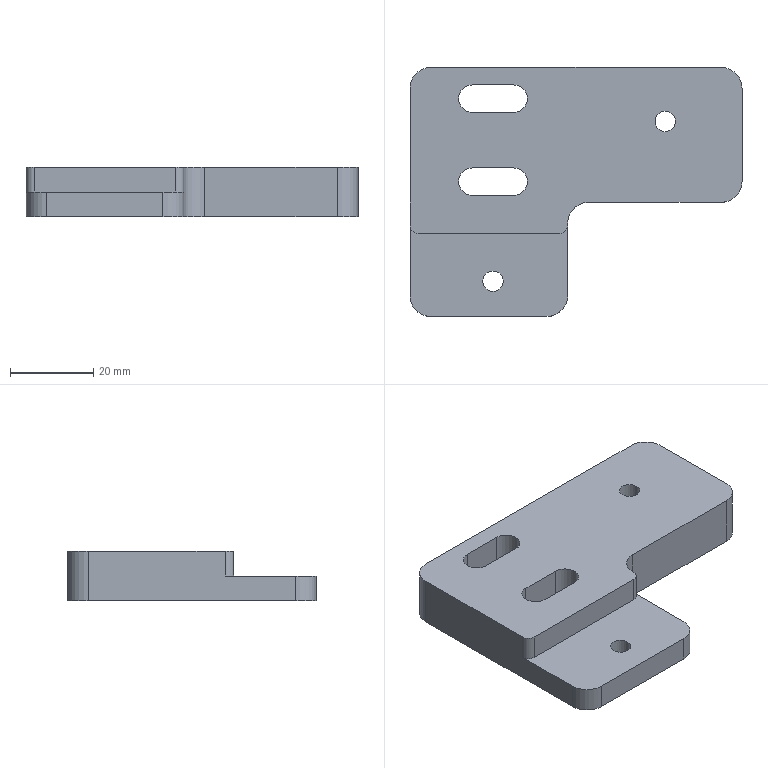NC program | NX | posted with a generic post | part box 80 x 60 x 12 mm
Lines 2097 to 2921 of 5338:
(ZLEVEL_PROFILE , TOOL : D4)
N4168 T11 M6
N4170 G54
N4172 G17 G0 G90 X-14.065 Y21.599 S9500 M3
N4174 G43 Z30. H11
N4176 Z1.5
N4178 G94 G1 X-13.892 Y21.801 Z1.486 F1650.
N4180 X-13.737 Y22.152 Z1.466
N4182 X-13.69 Y22.534 Z1.446
N4184 X-13.757 Y22.913 Z1.426
N4186 X-13.896 Y23.205 Z1.409
N4188 X-14.146 Y23.494 Z1.389
N4190 X-14.47 Y23.698 Z1.369
N4192 X-14.838 Y23.8 Z1.349
N4194 X-25.162 Z0.808
N4196 X-25.53 Y23.698 Z0.787
N4198 X-25.854 Y23.494 Z0.767
N4200 X-26.104 Y23.205 Z0.747
N4202 X-26.243 Y22.913 Z0.73
N4204 X-26.31 Y22.534 Z0.71
N4206 X-26.263 Y22.152 Z0.69
N4208 X-26.108 Y21.801 Z0.67
N4210 X-25.857 Y21.509 Z0.65
N4212 X-25.532 Y21.303 Z0.63
N4214 X-25.162 Y21.2 Z0.61
N4216 X-14.838 Z0.069
N4218 X-14.468 Y21.303 Z0.048
N4220 X-14.143 Y21.509 Z0.028
N4222 X-13.892 Y21.801 Z0.008
N4224 X-13.737 Y22.152 Z-0.012
N4226 X-13.69 Y22.534 Z-0.032
N4228 X-13.757 Y22.913 Z-0.052
N4230 X-13.896 Y23.205 Z-0.069
N4232 X-14.146 Y23.494 Z-0.089
N4234 X-14.47 Y23.698 Z-0.109
N4236 X-14.838 Y23.8 Z-0.129
N4238 X-20. Z-0.4
N4240 X-25.
N4242 G3 X-26.3 Y22.5 R1.3
N4244 X-25. Y21.2 R1.3
N4246 G1 X-15.
N4248 G3 X-13.7 Y22.5 R1.3
N4250 X-15. Y23.8 R1.3
N4252 G1 X-20.
N4254 X-24.789 Z-0.491
N4256 X-24.929 Z-0.493
N4258 X-25.07 Y23.79 Z-0.496
N4260 X-25.209 Y23.777 Z-0.499
N4262 X-25.346 Y23.746 Z-0.501
N4264 X-25.5 Y23.692 Z-0.504
N4266 X-25.606 Y23.643 Z-0.507
N4268 X-25.697 Y23.589 Z-0.509
N4270 X-25.742 Y23.562 Z-0.51
N4272 X-25.837 Y23.486 Z-0.512
N4274 X-25.963 Y23.362 Z-0.515
N4276 X-26.03 Y23.283 Z-0.517
N4278 X-26.113 Y23.162 Z-0.52
N4280 X-26.173 Y23.043 Z-0.523
N4282 X-26.238 Y22.871 Z-0.526
N4284 X-26.265 Y22.778 Z-0.528
N4286 X-26.286 Y22.637 Z-0.531
N4288 X-26.292 Y22.5 Z-0.533
N4290 X-26.28 Y22.323 Z-0.537
N4292 X-26.265 Y22.222 Z-0.539
N4294 X-26.224 Y22.085 Z-0.541
N4296 X-26.173 Y21.957 Z-0.544
N4298 X-26.093 Y21.809 Z-0.547
N4300 X-26.03 Y21.717 Z-0.549
N4302 X-25.925 Y21.598 Z-0.552
N4304 X-25.837 Y21.514 Z-0.555
N4306 X-25.709 Y21.417 Z-0.558
N4308 X-25.606 Y21.357 Z-0.56
N4310 X-25.452 Y21.289 Z-0.563
N4312 X-25.346 Y21.254 Z-0.565
N4314 X-25.209 Y21.223 Z-0.568
N4316 X-25.07 Y21.21 Z-0.571
N4318 X-24.929 Y21.2 Z-0.573
N4320 X-24.789 Z-0.576
N4322 X-15.211 Z-0.757
N4324 X-15.071 Z-0.76
N4326 X-14.93 Y21.21 Z-0.763
N4328 X-14.791 Y21.223 Z-0.765
N4330 X-14.654 Y21.254 Z-0.768
N4332 X-14.48 Y21.308 Z-0.771
N4334 X-14.391 Y21.351 Z-0.773
N4336 X-14.158 Y21.509 Z-0.779
N4338 X-14.094 Y21.568 Z-0.78
N4340 X-14.029 Y21.635 Z-0.782
N4342 X-13.97 Y21.717 Z-0.784
N4344 X-13.891 Y21.832 Z-0.787
N4346 X-13.827 Y21.957 Z-0.789
N4348 X-13.765 Y22.119 Z-0.793
N4350 X-13.735 Y22.222 Z-0.795
N4352 X-13.714 Y22.36 Z-0.797
N4354 X-13.7 Y22.5 Z-0.8
N4356 G3 X-15. Y23.8 R1.3
N4358 G1 X-20.
N4360 X-24.789 Z-0.891
N4362 X-24.929 Z-0.893
N4364 X-25.07 Y23.79 Z-0.896
N4366 X-25.209 Y23.777 Z-0.899
N4368 X-25.346 Y23.746 Z-0.901
N4370 X-25.5 Y23.692 Z-0.904
N4372 X-25.606 Y23.643 Z-0.907
N4374 X-25.697 Y23.589 Z-0.909
N4376 X-25.742 Y23.562 Z-0.91
N4378 X-25.837 Y23.486 Z-0.912
N4380 X-25.963 Y23.362 Z-0.915
N4382 X-26.03 Y23.283 Z-0.917
N4384 X-26.113 Y23.162 Z-0.92
N4386 X-26.173 Y23.043 Z-0.923
N4388 X-26.238 Y22.871 Z-0.926
N4390 X-26.265 Y22.778 Z-0.928
N4392 X-26.286 Y22.637 Z-0.931
N4394 X-26.292 Y22.5 Z-0.933
N4396 X-26.28 Y22.323 Z-0.937
N4398 X-26.265 Y22.222 Z-0.939
N4400 X-26.224 Y22.085 Z-0.941
N4402 X-26.173 Y21.957 Z-0.944
N4404 X-26.093 Y21.809 Z-0.947
N4406 X-26.03 Y21.717 Z-0.949
N4408 X-25.925 Y21.598 Z-0.952
N4410 X-25.837 Y21.514 Z-0.955
N4412 X-25.709 Y21.417 Z-0.958
N4414 X-25.606 Y21.357 Z-0.96
N4416 X-25.452 Y21.289 Z-0.963
N4418 X-25.346 Y21.254 Z-0.965
N4420 X-25.209 Y21.223 Z-0.968
N4422 X-25.07 Y21.21 Z-0.971
N4424 X-24.929 Y21.2 Z-0.973
N4426 X-24.789 Z-0.976
N4428 X-15.211 Z-1.157
N4430 X-15.071 Z-1.16
N4432 X-14.93 Y21.21 Z-1.163
N4434 X-14.791 Y21.223 Z-1.165
N4436 X-14.654 Y21.254 Z-1.168
N4438 X-14.48 Y21.308 Z-1.171
N4440 X-14.391 Y21.351 Z-1.173
N4442 X-14.158 Y21.509 Z-1.179
N4444 X-14.094 Y21.568 Z-1.18
N4446 X-14.029 Y21.635 Z-1.182
N4448 X-13.97 Y21.717 Z-1.184
N4450 X-13.891 Y21.832 Z-1.187
N4452 X-13.827 Y21.957 Z-1.189
N4454 X-13.765 Y22.119 Z-1.193
N4456 X-13.735 Y22.222 Z-1.195
N4458 X-13.714 Y22.36 Z-1.197
N4460 X-13.7 Y22.5 Z-1.2
N4462 G3 X-15. Y23.8 R1.3
N4464 G1 X-20.
N4466 X-24.789 Z-1.291
N4468 X-24.929 Z-1.293
N4470 X-25.07 Y23.79 Z-1.296
N4472 X-25.209 Y23.777 Z-1.299
N4474 X-25.346 Y23.746 Z-1.301
N4476 X-25.5 Y23.692 Z-1.304
N4478 X-25.606 Y23.643 Z-1.307
N4480 X-25.697 Y23.589 Z-1.309
N4482 X-25.742 Y23.562 Z-1.31
N4484 X-25.837 Y23.486 Z-1.312
N4486 X-25.962 Y23.362 Z-1.315
N4488 X-26.03 Y23.283 Z-1.317
N4490 X-26.113 Y23.162 Z-1.32
N4492 X-26.173 Y23.043 Z-1.323
N4494 X-26.238 Y22.871 Z-1.326
N4496 X-26.265 Y22.778 Z-1.328
N4498 X-26.286 Y22.637 Z-1.331
N4500 X-26.292 Y22.5 Z-1.333
N4502 X-26.28 Y22.323 Z-1.337
N4504 X-26.265 Y22.222 Z-1.339
N4506 X-26.224 Y22.085 Z-1.341
N4508 X-26.173 Y21.957 Z-1.344
N4510 X-26.093 Y21.809 Z-1.347
N4512 X-26.03 Y21.717 Z-1.349
N4514 X-25.925 Y21.598 Z-1.352
N4516 X-25.837 Y21.514 Z-1.355
N4518 X-25.709 Y21.417 Z-1.358
N4520 X-25.606 Y21.357 Z-1.36
N4522 X-25.452 Y21.289 Z-1.363
N4524 X-25.346 Y21.254 Z-1.365
N4526 X-25.209 Y21.223 Z-1.368
N4528 X-25.07 Y21.21 Z-1.371
N4530 X-24.929 Y21.2 Z-1.373
N4532 X-24.789 Z-1.376
N4534 X-15.211 Z-1.557
N4536 X-15.071 Z-1.56
N4538 X-14.93 Y21.21 Z-1.563
N4540 X-14.791 Y21.223 Z-1.565
N4542 X-14.654 Y21.254 Z-1.568
N4544 X-14.48 Y21.308 Z-1.571
N4546 X-14.391 Y21.351 Z-1.573
N4548 X-14.158 Y21.509 Z-1.579
N4550 X-14.094 Y21.568 Z-1.58
N4552 X-14.029 Y21.635 Z-1.582
N4554 X-13.97 Y21.717 Z-1.584
N4556 X-13.891 Y21.832 Z-1.587
N4558 X-13.827 Y21.957 Z-1.589
N4560 X-13.765 Y22.119 Z-1.593
N4562 X-13.735 Y22.222 Z-1.595
N4564 X-13.714 Y22.36 Z-1.597
N4566 X-13.7 Y22.5 Z-1.6
N4568 G3 X-15. Y23.8 R1.3
N4570 G1 X-20.
N4572 X-24.789 Z-1.691
N4574 X-24.929 Z-1.693
N4576 X-25.07 Y23.79 Z-1.696
N4578 X-25.209 Y23.777 Z-1.699
N4580 X-25.346 Y23.746 Z-1.701
N4582 X-25.5 Y23.692 Z-1.704
N4584 X-25.606 Y23.643 Z-1.707
N4586 X-25.697 Y23.589 Z-1.709
N4588 X-25.742 Y23.562 Z-1.71
N4590 X-25.837 Y23.486 Z-1.712
N4592 X-25.962 Y23.362 Z-1.715
N4594 X-26.03 Y23.283 Z-1.717
N4596 X-26.113 Y23.162 Z-1.72
N4598 X-26.173 Y23.043 Z-1.723
N4600 X-26.238 Y22.871 Z-1.726
N4602 X-26.265 Y22.778 Z-1.728
N4604 X-26.286 Y22.637 Z-1.731
N4606 X-26.292 Y22.5 Z-1.733
N4608 X-26.28 Y22.323 Z-1.737
N4610 X-26.265 Y22.222 Z-1.739
N4612 X-26.224 Y22.085 Z-1.741
N4614 X-26.173 Y21.957 Z-1.744
N4616 X-26.093 Y21.809 Z-1.747
N4618 X-26.03 Y21.717 Z-1.749
N4620 X-25.925 Y21.598 Z-1.752
N4622 X-25.837 Y21.514 Z-1.755
N4624 X-25.709 Y21.417 Z-1.758
N4626 X-25.606 Y21.357 Z-1.76
N4628 X-25.452 Y21.289 Z-1.763
N4630 X-25.346 Y21.254 Z-1.765
N4632 X-25.209 Y21.223 Z-1.768
N4634 X-25.07 Y21.21 Z-1.771
N4636 X-24.929 Y21.2 Z-1.773
N4638 X-24.789 Z-1.776
N4640 X-15.211 Z-1.957
N4642 X-15.071 Z-1.96
N4644 X-14.93 Y21.21 Z-1.963
N4646 X-14.791 Y21.223 Z-1.965
N4648 X-14.654 Y21.254 Z-1.968
N4650 X-14.48 Y21.308 Z-1.971
N4652 X-14.391 Y21.351 Z-1.973
N4654 X-14.158 Y21.509 Z-1.979
N4656 X-14.094 Y21.568 Z-1.98
N4658 X-14.029 Y21.635 Z-1.982
N4660 X-13.97 Y21.717 Z-1.984
N4662 X-13.891 Y21.832 Z-1.987
N4664 X-13.827 Y21.957 Z-1.989
N4666 X-13.765 Y22.119 Z-1.993
N4668 X-13.735 Y22.222 Z-1.995
N4670 X-13.714 Y22.36 Z-1.997
N4672 X-13.7 Y22.5 Z-2.
N4674 G3 X-15. Y23.8 R1.3
N4676 G1 X-20.
N4678 X-24.789 Z-2.091
N4680 X-24.929 Z-2.093
N4682 X-25.07 Y23.79 Z-2.096
N4684 X-25.209 Y23.777 Z-2.099
N4686 X-25.346 Y23.746 Z-2.101
N4688 X-25.5 Y23.692 Z-2.104
N4690 X-25.606 Y23.643 Z-2.107
N4692 X-25.697 Y23.589 Z-2.109
N4694 X-25.742 Y23.562 Z-2.11
N4696 X-25.837 Y23.486 Z-2.112
N4698 X-25.962 Y23.362 Z-2.115
N4700 X-26.03 Y23.283 Z-2.117
N4702 X-26.113 Y23.162 Z-2.12
N4704 X-26.173 Y23.043 Z-2.123
N4706 X-26.238 Y22.871 Z-2.126
N4708 X-26.265 Y22.778 Z-2.128
N4710 X-26.286 Y22.637 Z-2.131
N4712 X-26.292 Y22.5 Z-2.133
N4714 X-26.28 Y22.323 Z-2.137
N4716 X-26.265 Y22.222 Z-2.139
N4718 X-26.224 Y22.085 Z-2.141
N4720 X-26.173 Y21.957 Z-2.144
N4722 X-26.093 Y21.809 Z-2.147
N4724 X-26.03 Y21.717 Z-2.149
N4726 X-25.925 Y21.598 Z-2.152
N4728 X-25.837 Y21.514 Z-2.155
N4730 X-25.709 Y21.417 Z-2.158
N4732 X-25.606 Y21.357 Z-2.16
N4734 X-25.452 Y21.289 Z-2.163
N4736 X-25.346 Y21.254 Z-2.165
N4738 X-25.209 Y21.223 Z-2.168
N4740 X-25.07 Y21.21 Z-2.171
N4742 X-24.929 Y21.2 Z-2.173
N4744 X-24.789 Z-2.176
N4746 X-15.211 Z-2.357
N4748 X-15.071 Z-2.36
N4750 X-14.93 Y21.21 Z-2.363
N4752 X-14.791 Y21.223 Z-2.365
N4754 X-14.654 Y21.254 Z-2.368
N4756 X-14.48 Y21.308 Z-2.371
N4758 X-14.391 Y21.351 Z-2.373
N4760 X-14.158 Y21.509 Z-2.379
N4762 X-14.094 Y21.568 Z-2.38
N4764 X-14.03 Y21.635 Z-2.382
N4766 X-13.97 Y21.717 Z-2.384
N4768 X-13.891 Y21.832 Z-2.387
N4770 X-13.827 Y21.957 Z-2.389
N4772 X-13.765 Y22.119 Z-2.393
N4774 X-13.735 Y22.222 Z-2.395
N4776 X-13.714 Y22.36 Z-2.397
N4778 X-13.7 Y22.5 Z-2.4
N4780 G3 X-15. Y23.8 R1.3
N4782 G1 X-20.
N4784 X-24.789 Z-2.491
N4786 X-24.929 Z-2.493
N4788 X-25.07 Y23.79 Z-2.496
N4790 X-25.209 Y23.777 Z-2.499
N4792 X-25.346 Y23.746 Z-2.501
N4794 X-25.5 Y23.692 Z-2.504
N4796 X-25.606 Y23.643 Z-2.507
N4798 X-25.697 Y23.589 Z-2.509
N4800 X-25.742 Y23.562 Z-2.51
N4802 X-25.837 Y23.486 Z-2.512
N4804 X-25.962 Y23.362 Z-2.515
N4806 X-26.03 Y23.283 Z-2.517
N4808 X-26.113 Y23.162 Z-2.52
N4810 X-26.173 Y23.043 Z-2.523
N4812 X-26.238 Y22.871 Z-2.526
N4814 X-26.265 Y22.778 Z-2.528
N4816 X-26.286 Y22.637 Z-2.531
N4818 X-26.292 Y22.5 Z-2.533
N4820 X-26.28 Y22.323 Z-2.537
N4822 X-26.265 Y22.222 Z-2.539
N4824 X-26.224 Y22.085 Z-2.541
N4826 X-26.173 Y21.957 Z-2.544
N4828 X-26.093 Y21.809 Z-2.547
N4830 X-26.03 Y21.717 Z-2.549
N4832 X-25.925 Y21.598 Z-2.552
N4834 X-25.837 Y21.514 Z-2.555
N4836 X-25.709 Y21.417 Z-2.558
N4838 X-25.606 Y21.357 Z-2.56
N4840 X-25.452 Y21.289 Z-2.563
N4842 X-25.346 Y21.254 Z-2.565
N4844 X-25.209 Y21.223 Z-2.568
N4846 X-25.07 Y21.21 Z-2.571
N4848 X-24.929 Y21.2 Z-2.573
N4850 X-24.789 Z-2.576
N4852 X-15.211 Z-2.757
N4854 X-15.071 Z-2.76
N4856 X-14.93 Y21.21 Z-2.763
N4858 X-14.791 Y21.223 Z-2.765
N4860 X-14.654 Y21.254 Z-2.768
N4862 X-14.48 Y21.308 Z-2.771
N4864 X-14.391 Y21.351 Z-2.773
N4866 X-14.158 Y21.509 Z-2.779
N4868 X-14.094 Y21.567 Z-2.78
N4870 X-14.03 Y21.635 Z-2.782
N4872 X-13.97 Y21.717 Z-2.784
N4874 X-13.891 Y21.832 Z-2.787
N4876 X-13.827 Y21.957 Z-2.789
N4878 X-13.765 Y22.119 Z-2.793
N4880 X-13.735 Y22.222 Z-2.795
N4882 X-13.714 Y22.36 Z-2.797
N4884 X-13.7 Y22.5 Z-2.8
N4886 G3 X-15. Y23.8 R1.3
N4888 G1 X-20.
N4890 X-24.789 Z-2.891
N4892 X-24.929 Z-2.893
N4894 X-25.07 Y23.79 Z-2.896
N4896 X-25.209 Y23.777 Z-2.899
N4898 X-25.346 Y23.746 Z-2.901
N4900 X-25.5 Y23.692 Z-2.904
N4902 X-25.606 Y23.643 Z-2.907
N4904 X-25.742 Y23.562 Z-2.91
N4906 X-25.837 Y23.486 Z-2.912
N4908 X-25.962 Y23.362 Z-2.915
N4910 X-26.03 Y23.283 Z-2.917
N4912 X-26.113 Y23.162 Z-2.92
N4914 X-26.173 Y23.043 Z-2.923
N4916 X-26.238 Y22.871 Z-2.926
N4918 X-26.265 Y22.778 Z-2.928
N4920 X-26.286 Y22.637 Z-2.931
N4922 X-26.292 Y22.5 Z-2.933
N4924 X-26.28 Y22.323 Z-2.937
N4926 X-26.265 Y22.222 Z-2.939
N4928 X-26.224 Y22.085 Z-2.941
N4930 X-26.173 Y21.957 Z-2.944
N4932 X-26.093 Y21.809 Z-2.947
N4934 X-26.03 Y21.717 Z-2.949
N4936 X-25.925 Y21.598 Z-2.952
N4938 X-25.837 Y21.514 Z-2.955
N4940 X-25.709 Y21.417 Z-2.958
N4942 X-25.606 Y21.357 Z-2.96
N4944 X-25.452 Y21.289 Z-2.963
N4946 X-25.346 Y21.254 Z-2.965
N4948 X-25.209 Y21.223 Z-2.968
N4950 X-25.07 Y21.21 Z-2.971
N4952 X-24.929 Y21.2 Z-2.973
N4954 X-24.789 Z-2.976
N4956 X-15.211 Z-3.157
N4958 X-15.071 Z-3.16
N4960 X-14.93 Y21.21 Z-3.163
N4962 X-14.791 Y21.223 Z-3.165
N4964 X-14.654 Y21.254 Z-3.168
N4966 X-14.48 Y21.308 Z-3.171
N4968 X-14.391 Y21.351 Z-3.173
N4970 X-14.158 Y21.509 Z-3.179
N4972 X-14.094 Y21.567 Z-3.18
N4974 X-14.03 Y21.635 Z-3.182
N4976 X-13.97 Y21.717 Z-3.184
N4978 X-13.891 Y21.832 Z-3.187
N4980 X-13.827 Y21.957 Z-3.189
N4982 X-13.765 Y22.119 Z-3.193
N4984 X-13.735 Y22.222 Z-3.195
N4986 X-13.714 Y22.36 Z-3.197
N4988 X-13.7 Y22.5 Z-3.2
N4990 G3 X-15. Y23.8 R1.3
N4992 G1 X-20.
N4994 X-24.789 Z-3.291
N4996 X-24.929 Z-3.293
N4998 X-25.07 Y23.79 Z-3.296
N5000 X-25.209 Y23.777 Z-3.299
N5002 X-25.346 Y23.746 Z-3.301
N5004 X-25.5 Y23.692 Z-3.304
N5006 X-25.606 Y23.643 Z-3.307
N5008 X-25.742 Y23.562 Z-3.31
N5010 X-25.837 Y23.486 Z-3.312
N5012 X-25.962 Y23.362 Z-3.315
N5014 X-26.03 Y23.283 Z-3.317
N5016 X-26.113 Y23.162 Z-3.32
N5018 X-26.173 Y23.043 Z-3.323
N5020 X-26.238 Y22.871 Z-3.326
N5022 X-26.265 Y22.778 Z-3.328
N5024 X-26.286 Y22.638 Z-3.331
N5026 X-26.292 Y22.5 Z-3.333
N5028 X-26.28 Y22.323 Z-3.337
N5030 X-26.265 Y22.222 Z-3.339
N5032 X-26.224 Y22.085 Z-3.341
N5034 X-26.173 Y21.957 Z-3.344
N5036 X-26.093 Y21.809 Z-3.347
N5038 X-26.03 Y21.717 Z-3.349
N5040 X-25.925 Y21.598 Z-3.352
N5042 X-25.837 Y21.514 Z-3.355
N5044 X-25.709 Y21.417 Z-3.358
N5046 X-25.606 Y21.357 Z-3.36
N5048 X-25.452 Y21.289 Z-3.363
N5050 X-25.346 Y21.254 Z-3.365
N5052 X-25.209 Y21.223 Z-3.368
N5054 X-25.07 Y21.21 Z-3.371
N5056 X-24.929 Y21.2 Z-3.373
N5058 X-24.789 Z-3.376
N5060 X-15.211 Z-3.557
N5062 X-15.071 Z-3.56
N5064 X-14.93 Y21.21 Z-3.563
N5066 X-14.791 Y21.223 Z-3.565
N5068 X-14.654 Y21.254 Z-3.568
N5070 X-14.48 Y21.308 Z-3.571
N5072 X-14.391 Y21.351 Z-3.573
N5074 X-14.158 Y21.509 Z-3.579
N5076 X-14.094 Y21.567 Z-3.58
N5078 X-14.03 Y21.635 Z-3.582
N5080 X-13.97 Y21.717 Z-3.584
N5082 X-13.891 Y21.832 Z-3.587
N5084 X-13.827 Y21.957 Z-3.589
N5086 X-13.765 Y22.119 Z-3.593
N5088 X-13.735 Y22.222 Z-3.595
N5090 X-13.714 Y22.36 Z-3.597
N5092 X-13.7 Y22.5 Z-3.6
N5094 G3 X-15. Y23.8 R1.3
N5096 G1 X-20.
N5098 X-24.789 Z-3.691
N5100 X-24.929 Z-3.693
N5102 X-25.07 Y23.79 Z-3.696
N5104 X-25.209 Y23.777 Z-3.699
N5106 X-25.346 Y23.746 Z-3.701
N5108 X-25.5 Y23.692 Z-3.704
N5110 X-25.606 Y23.643 Z-3.707
N5112 X-25.742 Y23.562 Z-3.71
N5114 X-25.837 Y23.486 Z-3.712
N5116 X-25.962 Y23.362 Z-3.715
N5118 X-26.03 Y23.283 Z-3.717
N5120 X-26.113 Y23.162 Z-3.72
N5122 X-26.173 Y23.043 Z-3.723
N5124 X-26.238 Y22.871 Z-3.726
N5126 X-26.265 Y22.778 Z-3.728
N5128 X-26.286 Y22.638 Z-3.731
N5130 X-26.292 Y22.5 Z-3.733
N5132 X-26.28 Y22.324 Z-3.737
N5134 X-26.265 Y22.222 Z-3.739
N5136 X-26.224 Y22.085 Z-3.741
N5138 X-26.173 Y21.957 Z-3.744
N5140 X-26.093 Y21.809 Z-3.747
N5142 X-26.03 Y21.717 Z-3.749
N5144 X-25.925 Y21.598 Z-3.752
N5146 X-25.837 Y21.514 Z-3.755
N5148 X-25.709 Y21.417 Z-3.758
N5150 X-25.606 Y21.357 Z-3.76
N5152 X-25.452 Y21.289 Z-3.763
N5154 X-25.346 Y21.254 Z-3.765
N5156 X-25.209 Y21.223 Z-3.768
N5158 X-25.07 Y21.21 Z-3.771
N5160 X-24.929 Y21.2 Z-3.773
N5162 X-24.789 Z-3.776
N5164 X-15.211 Z-3.957
N5166 X-15.071 Z-3.96
N5168 X-14.93 Y21.21 Z-3.963
N5170 X-14.791 Y21.223 Z-3.965
N5172 X-14.654 Y21.254 Z-3.968
N5174 X-14.48 Y21.308 Z-3.971
N5176 X-14.391 Y21.351 Z-3.973
N5178 X-14.158 Y21.509 Z-3.979
N5180 X-14.094 Y21.567 Z-3.98
N5182 X-14.03 Y21.635 Z-3.982
N5184 X-13.97 Y21.717 Z-3.984
N5186 X-13.891 Y21.832 Z-3.987
N5188 X-13.827 Y21.957 Z-3.989
N5190 X-13.766 Y22.119 Z-3.993
N5192 X-13.735 Y22.222 Z-3.995
N5194 X-13.714 Y22.36 Z-3.997
N5196 X-13.7 Y22.5 Z-4.
N5198 G3 X-15. Y23.8 R1.3
N5200 G1 X-20.
N5202 X-24.789 Z-4.091
N5204 X-24.929 Z-4.093
N5206 X-25.07 Y23.79 Z-4.096
N5208 X-25.209 Y23.777 Z-4.099
N5210 X-25.346 Y23.746 Z-4.101
N5212 X-25.5 Y23.692 Z-4.104
N5214 X-25.606 Y23.643 Z-4.107
N5216 X-25.742 Y23.562 Z-4.11
N5218 X-25.837 Y23.486 Z-4.112
N5220 X-25.962 Y23.362 Z-4.115
N5222 X-26.03 Y23.283 Z-4.117
N5224 X-26.113 Y23.162 Z-4.12
N5226 X-26.173 Y23.043 Z-4.123
N5228 X-26.238 Y22.871 Z-4.126
N5230 X-26.265 Y22.778 Z-4.128
N5232 X-26.286 Y22.638 Z-4.131
N5234 X-26.292 Y22.5 Z-4.133
N5236 X-26.28 Y22.324 Z-4.137
N5238 X-26.265 Y22.222 Z-4.139
N5240 X-26.224 Y22.085 Z-4.141
N5242 X-26.173 Y21.957 Z-4.144
N5244 X-26.093 Y21.809 Z-4.147
N5246 X-26.03 Y21.717 Z-4.149
N5248 X-25.925 Y21.598 Z-4.152
N5250 X-25.837 Y21.514 Z-4.155
N5252 X-25.709 Y21.417 Z-4.158
N5254 X-25.606 Y21.357 Z-4.16
N5256 X-25.452 Y21.289 Z-4.163
N5258 X-25.346 Y21.254 Z-4.165
N5260 X-25.209 Y21.223 Z-4.168
N5262 X-25.07 Y21.21 Z-4.171
N5264 X-24.929 Y21.2 Z-4.173
N5266 X-24.789 Z-4.176
N5268 X-15.211 Z-4.357
N5270 X-15.071 Z-4.36
N5272 X-14.93 Y21.21 Z-4.363
N5274 X-14.791 Y21.223 Z-4.365
N5276 X-14.654 Y21.254 Z-4.368
N5278 X-14.48 Y21.308 Z-4.371
N5280 X-14.391 Y21.351 Z-4.373
N5282 X-14.158 Y21.509 Z-4.379
N5284 X-14.094 Y21.567 Z-4.38
N5286 X-14.03 Y21.635 Z-4.382
N5288 X-13.97 Y21.717 Z-4.384
N5290 X-13.891 Y21.832 Z-4.387
N5292 X-13.827 Y21.957 Z-4.389
N5294 X-13.766 Y22.119 Z-4.393
N5296 X-13.735 Y22.222 Z-4.395
N5298 X-13.714 Y22.36 Z-4.397
N5300 X-13.7 Y22.5 Z-4.4
N5302 G3 X-15. Y23.8 R1.3
N5304 G1 X-20.
N5306 X-24.789 Z-4.491
N5308 X-24.929 Z-4.493
N5310 X-25.07 Y23.79 Z-4.496
N5312 X-25.209 Y23.777 Z-4.499
N5314 X-25.346 Y23.746 Z-4.501
N5316 X-25.5 Y23.692 Z-4.504
N5318 X-25.606 Y23.643 Z-4.507
N5320 X-25.742 Y23.562 Z-4.51
N5322 X-25.837 Y23.486 Z-4.512
N5324 X-25.962 Y23.362 Z-4.515
N5326 X-26.03 Y23.283 Z-4.517
N5328 X-26.113 Y23.162 Z-4.52
N5330 X-26.173 Y23.043 Z-4.523
N5332 X-26.238 Y22.871 Z-4.526
N5334 X-26.265 Y22.778 Z-4.528
N5336 X-26.286 Y22.638 Z-4.531
N5338 X-26.292 Y22.5 Z-4.533
N5340 X-26.28 Y22.324 Z-4.537
N5342 X-26.265 Y22.222 Z-4.539
N5344 X-26.224 Y22.085 Z-4.541
N5346 X-26.173 Y21.957 Z-4.544
N5348 X-26.093 Y21.809 Z-4.547
N5350 X-26.03 Y21.717 Z-4.549
N5352 X-25.925 Y21.598 Z-4.552
N5354 X-25.837 Y21.514 Z-4.555
N5356 X-25.709 Y21.417 Z-4.558
N5358 X-25.606 Y21.357 Z-4.56
N5360 X-25.452 Y21.289 Z-4.563
N5362 X-25.346 Y21.254 Z-4.565
N5364 X-25.209 Y21.223 Z-4.568
N5366 X-25.07 Y21.21 Z-4.571
N5368 X-24.929 Y21.2 Z-4.573
N5370 X-24.789 Z-4.576
N5372 X-15.211 Z-4.757
N5374 X-15.071 Z-4.76
N5376 X-14.93 Y21.21 Z-4.763
N5378 X-14.791 Y21.223 Z-4.765
N5380 X-14.654 Y21.254 Z-4.768
N5382 X-14.48 Y21.308 Z-4.771
N5384 X-14.391 Y21.351 Z-4.773
N5386 X-14.158 Y21.509 Z-4.779
N5388 X-14.094 Y21.567 Z-4.78
N5390 X-14.03 Y21.635 Z-4.782
N5392 X-13.97 Y21.717 Z-4.784
N5394 X-13.891 Y21.832 Z-4.787
N5396 X-13.827 Y21.957 Z-4.789
N5398 X-13.766 Y22.119 Z-4.793
N5400 X-13.735 Y22.222 Z-4.795
N5402 X-13.714 Y22.36 Z-4.797
N5404 X-13.7 Y22.5 Z-4.8
N5406 G3 X-15. Y23.8 R1.3
N5408 G1 X-20.
N5410 X-24.789 Z-4.891
N5412 X-24.929 Z-4.893
N5414 X-25.07 Y23.79 Z-4.896
N5416 X-25.209 Y23.777 Z-4.899
N5418 X-25.346 Y23.746 Z-4.901
N5420 X-25.5 Y23.692 Z-4.904
N5422 X-25.606 Y23.643 Z-4.907
N5424 X-25.742 Y23.562 Z-4.91
N5426 X-25.837 Y23.486 Z-4.912
N5428 X-25.962 Y23.362 Z-4.915
N5430 X-26.03 Y23.283 Z-4.917
N5432 X-26.113 Y23.162 Z-4.92
N5434 X-26.173 Y23.043 Z-4.923
N5436 X-26.238 Y22.871 Z-4.926
N5438 X-26.265 Y22.778 Z-4.928
N5440 X-26.286 Y22.638 Z-4.931
N5442 X-26.292 Y22.5 Z-4.933
N5444 X-26.28 Y22.324 Z-4.937
N5446 X-26.265 Y22.222 Z-4.939
N5448 X-26.224 Y22.085 Z-4.941
N5450 X-26.173 Y21.957 Z-4.944
N5452 X-26.093 Y21.809 Z-4.947
N5454 X-26.03 Y21.717 Z-4.949
N5456 X-25.925 Y21.598 Z-4.952
N5458 X-25.837 Y21.514 Z-4.955
N5460 X-25.709 Y21.417 Z-4.958
N5462 X-25.606 Y21.357 Z-4.96
N5464 X-25.452 Y21.289 Z-4.963
N5466 X-25.346 Y21.254 Z-4.965
N5468 X-25.209 Y21.223 Z-4.968
N5470 X-25.07 Y21.21 Z-4.971
N5472 X-24.929 Y21.2 Z-4.973
N5474 X-24.789 Z-4.976
N5476 X-15.211 Z-5.157
N5478 X-15.071 Z-5.16
N5480 X-14.93 Y21.21 Z-5.163
N5482 X-14.791 Y21.223 Z-5.165
N5484 X-14.654 Y21.254 Z-5.168
N5486 X-14.48 Y21.308 Z-5.171
N5488 X-14.391 Y21.351 Z-5.173
N5490 X-14.158 Y21.509 Z-5.179
N5492 X-14.094 Y21.567 Z-5.18
N5494 X-14.03 Y21.635 Z-5.182
N5496 X-13.97 Y21.717 Z-5.184
N5498 X-13.891 Y21.832 Z-5.187
N5500 X-13.827 Y21.957 Z-5.189
N5502 X-13.766 Y22.119 Z-5.193
N5504 X-13.735 Y22.222 Z-5.195
N5506 X-13.714 Y22.36 Z-5.197
N5508 X-13.7 Y22.5 Z-5.2
N5510 G3 X-15. Y23.8 R1.3
N5512 G1 X-20.
N5514 X-24.789 Z-5.291
N5516 X-24.929 Z-5.293
N5518 X-25.07 Y23.79 Z-5.296
N5520 X-25.209 Y23.777 Z-5.299
N5522 X-25.346 Y23.746 Z-5.301
N5524 X-25.5 Y23.692 Z-5.304
N5526 X-25.606 Y23.643 Z-5.307
N5528 X-25.742 Y23.562 Z-5.31
N5530 X-25.837 Y23.486 Z-5.312
N5532 X-25.962 Y23.362 Z-5.315
N5534 X-26.03 Y23.283 Z-5.317
N5536 X-26.113 Y23.162 Z-5.32
N5538 X-26.173 Y23.043 Z-5.323
N5540 X-26.238 Y22.871 Z-5.326
N5542 X-26.265 Y22.778 Z-5.328
N5544 X-26.286 Y22.638 Z-5.331
N5546 X-26.292 Y22.5 Z-5.333
N5548 X-26.28 Y22.324 Z-5.337
N5550 X-26.265 Y22.222 Z-5.339
N5552 X-26.224 Y22.085 Z-5.341
N5554 X-26.173 Y21.957 Z-5.344
N5556 X-26.093 Y21.809 Z-5.347
N5558 X-26.03 Y21.717 Z-5.349
N5560 X-25.925 Y21.598 Z-5.352
N5562 X-25.837 Y21.514 Z-5.355
N5564 X-25.709 Y21.417 Z-5.358
N5566 X-25.606 Y21.357 Z-5.36
N5568 X-25.452 Y21.289 Z-5.363
N5570 X-25.346 Y21.254 Z-5.365
N5572 X-25.209 Y21.223 Z-5.368
N5574 X-25.07 Y21.21 Z-5.371
N5576 X-24.929 Y21.2 Z-5.373
N5578 X-24.789 Z-5.376
N5580 X-15.211 Z-5.557
N5582 X-15.071 Z-5.56
N5584 X-14.93 Y21.21 Z-5.563
N5586 X-14.791 Y21.223 Z-5.565
N5588 X-14.654 Y21.254 Z-5.568
N5590 X-14.48 Y21.308 Z-5.571
N5592 X-14.391 Y21.351 Z-5.573
N5594 X-14.158 Y21.509 Z-5.579
N5596 X-14.094 Y21.567 Z-5.58
N5598 X-14.03 Y21.635 Z-5.582
N5600 X-13.97 Y21.717 Z-5.584
N5602 X-13.891 Y21.832 Z-5.587
N5604 X-13.827 Y21.957 Z-5.589
N5606 X-13.766 Y22.119 Z-5.593
N5608 X-13.735 Y22.222 Z-5.595
N5610 X-13.714 Y22.36 Z-5.597
N5612 X-13.7 Y22.5 Z-5.6
N5614 G3 X-15. Y23.8 R1.3
N5616 G1 X-20.
N5618 X-24.789 Z-5.691
N5620 X-24.929 Z-5.693
N5622 X-25.07 Y23.79 Z-5.696
N5624 X-25.209 Y23.777 Z-5.699
N5626 X-25.346 Y23.746 Z-5.701
N5628 X-25.5 Y23.691 Z-5.704
N5630 X-25.606 Y23.643 Z-5.707
N5632 X-25.742 Y23.562 Z-5.71
N5634 X-25.837 Y23.486 Z-5.712
N5636 X-25.962 Y23.362 Z-5.715
N5638 X-26.03 Y23.283 Z-5.717
N5640 X-26.113 Y23.162 Z-5.72
N5642 X-26.173 Y23.043 Z-5.723
N5644 X-26.238 Y22.871 Z-5.726
N5646 X-26.265 Y22.778 Z-5.728
N5648 X-26.286 Y22.638 Z-5.731
N5650 X-26.292 Y22.5 Z-5.733
N5652 X-26.28 Y22.324 Z-5.737
N5654 X-26.265 Y22.222 Z-5.739
N5656 X-26.224 Y22.085 Z-5.741
N5658 X-26.173 Y21.957 Z-5.744
N5660 X-26.093 Y21.809 Z-5.747
N5662 X-26.03 Y21.717 Z-5.749
N5664 X-25.925 Y21.598 Z-5.752
N5666 X-25.837 Y21.514 Z-5.755
N5668 X-25.709 Y21.417 Z-5.758
N5670 X-25.606 Y21.357 Z-5.76
N5672 X-25.452 Y21.289 Z-5.763
N5674 X-25.346 Y21.254 Z-5.765
N5676 X-25.209 Y21.223 Z-5.768
N5678 X-25.07 Y21.21 Z-5.771
N5680 X-24.929 Y21.2 Z-5.773
N5682 X-24.789 Z-5.776
N5684 X-15.211 Z-5.957
N5686 X-15.071 Z-5.96
N5688 X-14.93 Y21.21 Z-5.963
N5690 X-14.791 Y21.223 Z-5.965
N5692 X-14.654 Y21.254 Z-5.968
N5694 X-14.48 Y21.308 Z-5.971
N5696 X-14.391 Y21.351 Z-5.973
N5698 X-14.158 Y21.509 Z-5.979
N5700 X-14.094 Y21.567 Z-5.98
N5702 X-14.03 Y21.635 Z-5.982
N5704 X-13.97 Y21.717 Z-5.984
N5706 X-13.891 Y21.832 Z-5.987
N5708 X-13.827 Y21.957 Z-5.989
N5710 X-13.766 Y22.119 Z-5.993
N5712 X-13.735 Y22.222 Z-5.995
N5714 X-13.714 Y22.36 Z-5.997
N5716 X-13.7 Y22.5 Z-6.
N5718 G3 X-15. Y23.8 R1.3
N5720 G1 X-20.
N5722 X-24.789 Z-6.091
N5724 X-24.929 Z-6.093
N5726 X-25.07 Y23.79 Z-6.096
N5728 X-25.209 Y23.777 Z-6.099
N5730 X-25.346 Y23.746 Z-6.101
N5732 X-25.5 Y23.691 Z-6.104
N5734 X-25.606 Y23.643 Z-6.107
N5736 X-25.742 Y23.562 Z-6.11
N5738 X-25.837 Y23.486 Z-6.112
N5740 X-25.962 Y23.362 Z-6.115
N5742 X-26.03 Y23.283 Z-6.117
N5744 X-26.113 Y23.162 Z-6.12
N5746 X-26.173 Y23.043 Z-6.123
N5748 X-26.238 Y22.871 Z-6.126
N5750 X-26.265 Y22.778 Z-6.128
N5752 X-26.286 Y22.638 Z-6.131
N5754 X-26.292 Y22.5 Z-6.133
N5756 X-26.28 Y22.324 Z-6.137
N5758 X-26.265 Y22.222 Z-6.139
N5760 X-26.224 Y22.085 Z-6.141
N5762 X-26.173 Y21.957 Z-6.144
N5764 X-26.093 Y21.809 Z-6.147
N5766 X-26.03 Y21.717 Z-6.149
N5768 X-25.925 Y21.598 Z-6.152
N5770 X-25.837 Y21.514 Z-6.155
N5772 X-25.709 Y21.417 Z-6.158
N5774 X-25.606 Y21.357 Z-6.16
N5776 X-25.452 Y21.289 Z-6.163
N5778 X-25.346 Y21.254 Z-6.165
N5780 X-25.209 Y21.223 Z-6.168
N5782 X-25.07 Y21.21 Z-6.171
N5784 X-24.929 Y21.2 Z-6.173
N5786 X-24.789 Z-6.176
N5788 X-15.211 Z-6.357
N5790 X-15.071 Z-6.36
N5792 X-14.93 Y21.21 Z-6.363
N5794 X-14.791 Y21.223 Z-6.365
N5796 X-14.654 Y21.254 Z-6.368
N5798 X-14.48 Y21.308 Z-6.371
N5800 X-14.391 Y21.351 Z-6.373
N5802 X-14.158 Y21.509 Z-6.379
N5804 X-14.094 Y21.567 Z-6.38
N5806 X-14.03 Y21.635 Z-6.382
N5808 X-13.97 Y21.717 Z-6.384
N5810 X-13.891 Y21.832 Z-6.387